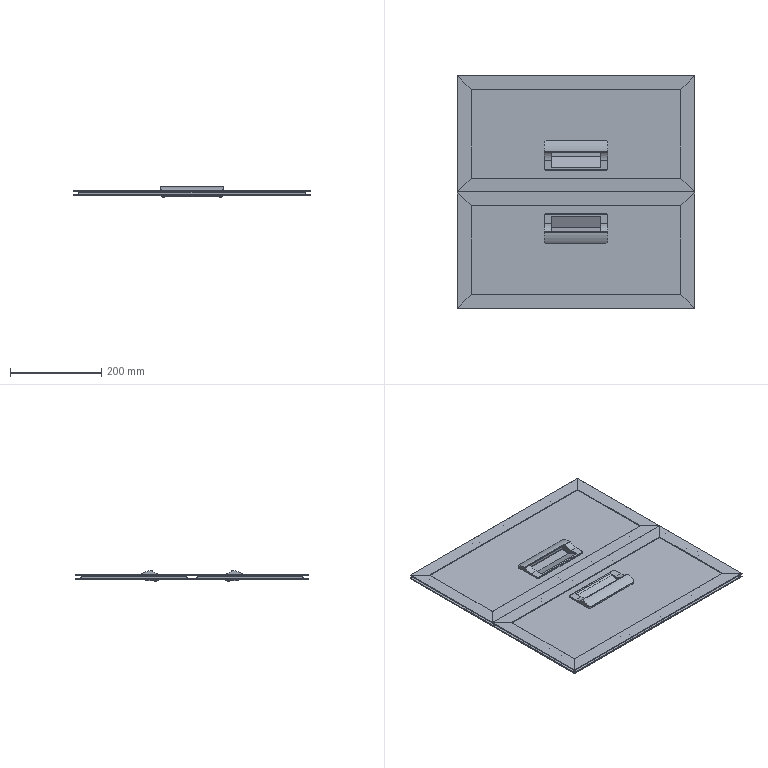Part | SolidWorks | 12 solids | 318 faces | box 520 x 510 x 23.592 mm | volume 1484589 mm3 | plane 206 | cylinder 88 | spline 8 | cone 8 | torus 8 | commonest cylinder face diameters 2 x44 4 x8 8 x8 10 x8 12 x8 52 x6